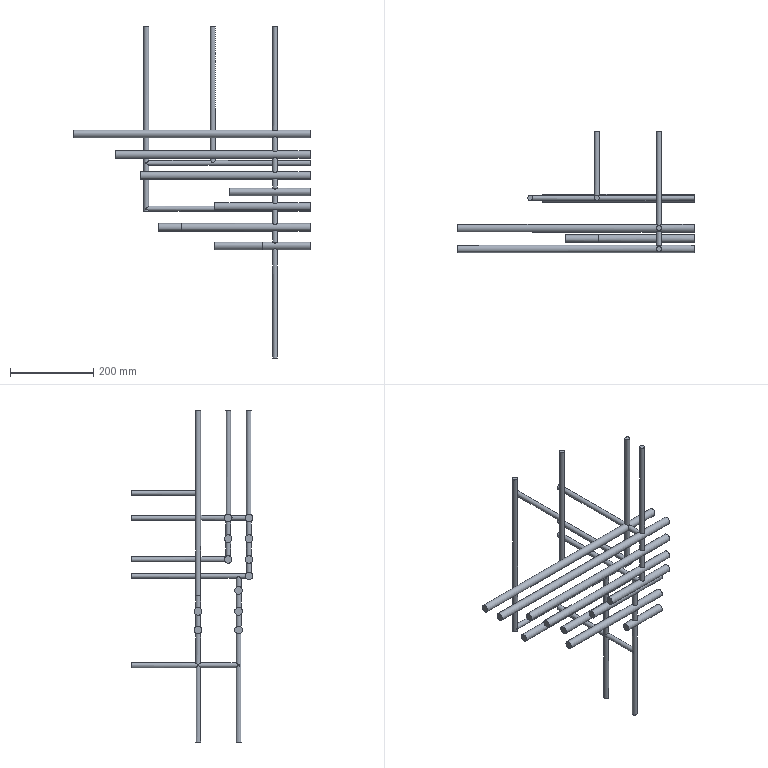Part | STEP file | solid 260 | 1 solid | 93 faces | box 570 x 292.75 x 800 mm | volume 1618507 mm3 | plane 47 | cylinder 46 | commonest cylinder face diameters 12 x34 18.5 x12